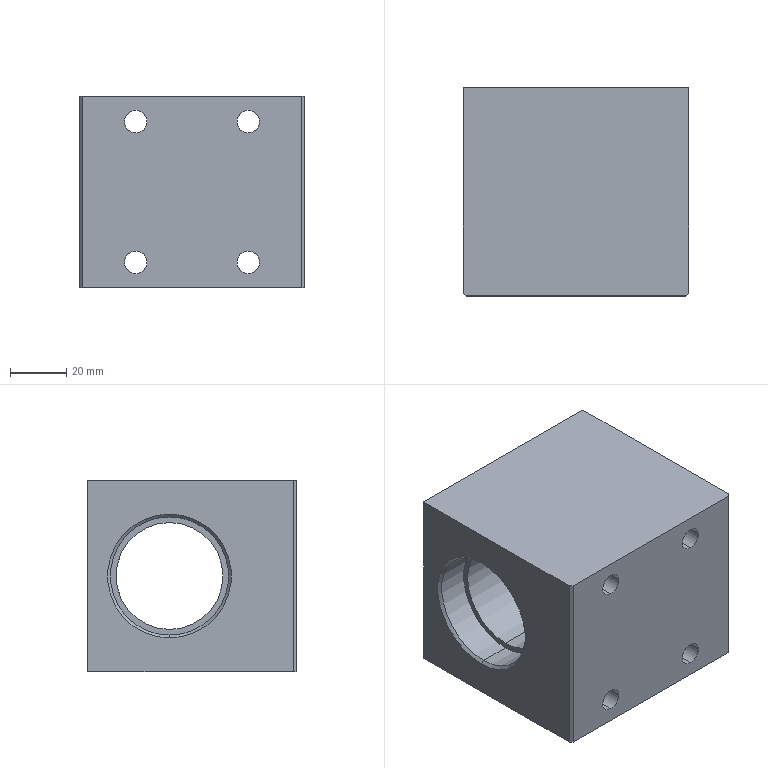Part | SolidWorks | features MirrorPattern 3, Chamfer 2, HoleWzd 2, ICE 2, Extrusion 1, MirrorSolid 1 | 1 solid | 42 faces | box 80 x 74 x 68 mm | volume 288342 mm3 | cylinder 24 | plane 14 | cone 4 | commonest cylinder face diameters 8 x8 12 x8 42 x4 6.8 x2 38 x2
STEP:
#1=CARTESIAN_POINT('',(20.,29.,19.));
#2=VERTEX_POINT('',#1);
#3=CARTESIAN_POINT('',(20.,29.,31.));
#4=VERTEX_POINT('',#3);
#5=CARTESIAN_POINT('',(20.,29.,25.));
#6=DIRECTION('',(0.,1.,0.));
#7=DIRECTION('',(0.,0.,1.));
#8=AXIS2_PLACEMENT_3D('',#5,#6,#7);
#9=CIRCLE('',#8,6.);
#10=EDGE_CURVE('',#2,#4,#9,.T.);
#11=ORIENTED_EDGE('',*,*,#10,.F.);
#12=CARTESIAN_POINT('',(20.,37.,19.));
#13=VERTEX_POINT('',#12);
#14=CARTESIAN_POINT('',(20.,37.,19.));
#15=DIRECTION('',(0.,1.,0.));
#16=VECTOR('',#15,1000.);
#17=LINE('',#14,#16);
#18=EDGE_CURVE('',#2,#13,#17,.T.);
#19=ORIENTED_EDGE('',*,*,#18,.T.);
#20=CARTESIAN_POINT('',(20.,37.,31.));
#21=VERTEX_POINT('',#20);
#22=CARTESIAN_POINT('',(20.,37.,25.));
#23=DIRECTION('',(0.,1.,0.));
#24=DIRECTION('',(0.,0.,1.));
#25=AXIS2_PLACEMENT_3D('',#22,#23,#24);
#26=CIRCLE('',#25,6.);
#27=EDGE_CURVE('',#13,#21,#26,.T.);
#28=ORIENTED_EDGE('',*,*,#27,.T.);
#29=CARTESIAN_POINT('',(20.,37.,31.));
#30=DIRECTION('',(0.,1.,0.));
#31=VECTOR('',#30,1000.);
#32=LINE('',#29,#31);
#33=EDGE_CURVE('',#4,#21,#32,.T.);
#34=ORIENTED_EDGE('',*,*,#33,.F.);
#35=EDGE_LOOP('',(#11,#19,#28,#34));
#36=FACE_OUTER_BOUND('',#35,.T.);
#37=CARTESIAN_POINT('',(20.,37.,25.));
#38=DIRECTION('',(0.,1.,0.));
#39=DIRECTION('',(0.,0.,1.));
#40=AXIS2_PLACEMENT_3D('',#37,#38,#39);
#41=CYLINDRICAL_SURFACE('',#40,6.);
#42=ADVANCED_FACE('',(#36),#41,.F.);
#43=CARTESIAN_POINT('',(20.,-37.,21.));
#44=VERTEX_POINT('',#43);
#45=CARTESIAN_POINT('',(20.,-37.,29.));
#46=VERTEX_POINT('',#45);
#47=CARTESIAN_POINT('',(20.,-37.,25.));
#48=DIRECTION('',(0.,1.,0.));
#49=DIRECTION('',(0.,0.,1.));
#50=AXIS2_PLACEMENT_3D('',#47,#48,#49);
#51=CIRCLE('',#50,4.);
#52=EDGE_CURVE('',#44,#46,#51,.T.);
#53=ORIENTED_EDGE('',*,*,#52,.F.);
#54=CARTESIAN_POINT('',(20.,29.,21.));
#55=VERTEX_POINT('',#54);
#56=CARTESIAN_POINT('',(20.,37.,21.));
#57=DIRECTION('',(0.,1.,0.));
#58=VECTOR('',#57,1000.);
#59=LINE('',#56,#58);
#60=EDGE_CURVE('',#44,#55,#59,.T.);
#61=ORIENTED_EDGE('',*,*,#60,.T.);
#62=CARTESIAN_POINT('',(20.,29.,29.));
#63=VERTEX_POINT('',#62);
#64=CARTESIAN_POINT('',(20.,29.,25.));
#65=DIRECTION('',(0.,1.,0.));
#66=DIRECTION('',(0.,0.,1.));
#67=AXIS2_PLACEMENT_3D('',#64,#65,#66);
#68=CIRCLE('',#67,4.);
#69=EDGE_CURVE('',#55,#63,#68,.T.);
#70=ORIENTED_EDGE('',*,*,#69,.T.);
#71=CARTESIAN_POINT('',(20.,37.,29.));
#72=DIRECTION('',(0.,1.,0.));
#73=VECTOR('',#72,1000.);
#74=LINE('',#71,#73);
#75=EDGE_CURVE('',#46,#63,#74,.T.);
#76=ORIENTED_EDGE('',*,*,#75,.F.);
#77=EDGE_LOOP('',(#53,#61,#70,#76));
#78=FACE_OUTER_BOUND('',#77,.T.);
#79=CARTESIAN_POINT('',(20.,37.,25.));
#80=DIRECTION('',(0.,1.,0.));
#81=DIRECTION('',(0.,0.,1.));
#82=AXIS2_PLACEMENT_3D('',#79,#80,#81);
#83=CYLINDRICAL_SURFACE('',#82,4.);
#84=ADVANCED_FACE('',(#78),#83,.F.);
#85=CARTESIAN_POINT('',(20.,29.,-31.));
#86=VERTEX_POINT('',#85);
#87=CARTESIAN_POINT('',(20.,29.,-19.));
#88=VERTEX_POINT('',#87);
#89=CARTESIAN_POINT('',(20.,29.,-25.));
#90=DIRECTION('',(0.,1.,0.));
#91=DIRECTION('',(0.,0.,1.));
#92=AXIS2_PLACEMENT_3D('',#89,#90,#91);
#93=CIRCLE('',#92,6.);
#94=EDGE_CURVE('',#86,#88,#93,.T.);
#95=ORIENTED_EDGE('',*,*,#94,.F.);
#96=CARTESIAN_POINT('',(20.,37.,-31.));
#97=VERTEX_POINT('',#96);
#98=CARTESIAN_POINT('',(20.,37.,-31.));
#99=DIRECTION('',(0.,1.,0.));
#100=VECTOR('',#99,1000.);
#101=LINE('',#98,#100);
#102=EDGE_CURVE('',#86,#97,#101,.T.);
#103=ORIENTED_EDGE('',*,*,#102,.T.);
#104=CARTESIAN_POINT('',(20.,37.,-19.));
#105=VERTEX_POINT('',#104);
#106=CARTESIAN_POINT('',(20.,37.,-25.));
#107=DIRECTION('',(0.,1.,0.));
#108=DIRECTION('',(0.,0.,1.));
#109=AXIS2_PLACEMENT_3D('',#106,#107,#108);
#110=CIRCLE('',#109,6.);
#111=EDGE_CURVE('',#97,#105,#110,.T.);
#112=ORIENTED_EDGE('',*,*,#111,.T.);
#113=CARTESIAN_POINT('',(20.,37.,-19.));
#114=DIRECTION('',(0.,1.,0.));
#115=VECTOR('',#114,1000.);
#116=LINE('',#113,#115);
#117=EDGE_CURVE('',#88,#105,#116,.T.);
#118=ORIENTED_EDGE('',*,*,#117,.F.);
#119=EDGE_LOOP('',(#95,#103,#112,#118));
#120=FACE_OUTER_BOUND('',#119,.T.);
#121=CARTESIAN_POINT('',(20.,37.,-25.));
#122=DIRECTION('',(0.,1.,0.));
#123=DIRECTION('',(0.,0.,1.));
#124=AXIS2_PLACEMENT_3D('',#121,#122,#123);
#125=CYLINDRICAL_SURFACE('',#124,6.);
#126=ADVANCED_FACE('',(#120),#125,.F.);
#127=CARTESIAN_POINT('',(20.,-37.,-29.));
#128=VERTEX_POINT('',#127);
#129=CARTESIAN_POINT('',(20.,-37.,-21.));
#130=VERTEX_POINT('',#129);
#131=CARTESIAN_POINT('',(20.,-37.,-25.));
#132=DIRECTION('',(0.,1.,0.));
#133=DIRECTION('',(0.,0.,1.));
#134=AXIS2_PLACEMENT_3D('',#131,#132,#133);
#135=CIRCLE('',#134,4.);
#136=EDGE_CURVE('',#128,#130,#135,.T.);
#137=ORIENTED_EDGE('',*,*,#136,.F.);
#138=CARTESIAN_POINT('',(20.,29.,-29.));
#139=VERTEX_POINT('',#138);
#140=CARTESIAN_POINT('',(20.,37.,-29.));
#141=DIRECTION('',(0.,1.,0.));
#142=VECTOR('',#141,1000.);
#143=LINE('',#140,#142);
#144=EDGE_CURVE('',#128,#139,#143,.T.);
#145=ORIENTED_EDGE('',*,*,#144,.T.);
#146=CARTESIAN_POINT('',(20.,29.,-21.));
#147=VERTEX_POINT('',#146);
#148=CARTESIAN_POINT('',(20.,29.,-25.));
#149=DIRECTION('',(0.,1.,0.));
#150=DIRECTION('',(0.,0.,1.));
#151=AXIS2_PLACEMENT_3D('',#148,#149,#150);
#152=CIRCLE('',#151,4.);
#153=EDGE_CURVE('',#139,#147,#152,.T.);
#154=ORIENTED_EDGE('',*,*,#153,.T.);
#155=CARTESIAN_POINT('',(20.,37.,-21.));
#156=DIRECTION('',(0.,1.,0.));
#157=VECTOR('',#156,1000.);
#158=LINE('',#155,#157);
#159=EDGE_CURVE('',#130,#147,#158,.T.);
#160=ORIENTED_EDGE('',*,*,#159,.F.);
#161=EDGE_LOOP('',(#137,#145,#154,#160));
#162=FACE_OUTER_BOUND('',#161,.T.);
#163=CARTESIAN_POINT('',(20.,37.,-25.));
#164=DIRECTION('',(0.,1.,0.));
#165=DIRECTION('',(0.,0.,1.));
#166=AXIS2_PLACEMENT_3D('',#163,#164,#165);
#167=CYLINDRICAL_SURFACE('',#166,4.);
#168=ADVANCED_FACE('',(#162),#167,.F.);
#169=CARTESIAN_POINT('',(-20.,29.,-31.));
#170=VERTEX_POINT('',#169);
#171=CARTESIAN_POINT('',(-20.,29.,-19.));
#172=VERTEX_POINT('',#171);
#173=CARTESIAN_POINT('',(-20.,29.,-25.));
#174=DIRECTION('',(0.,1.,0.));
#175=DIRECTION('',(0.,0.,1.));
#176=AXIS2_PLACEMENT_3D('',#173,#174,#175);
#177=CIRCLE('',#176,6.);
#178=EDGE_CURVE('',#170,#172,#177,.T.);
#179=ORIENTED_EDGE('',*,*,#178,.F.);
#180=CARTESIAN_POINT('',(-20.,37.,-31.));
#181=VERTEX_POINT('',#180);
#182=CARTESIAN_POINT('',(-20.,37.,-31.));
#183=DIRECTION('',(0.,1.,0.));
#184=VECTOR('',#183,1000.);
#185=LINE('',#182,#184);
#186=EDGE_CURVE('',#170,#181,#185,.T.);
#187=ORIENTED_EDGE('',*,*,#186,.T.);
#188=CARTESIAN_POINT('',(-20.,37.,-19.));
#189=VERTEX_POINT('',#188);
#190=CARTESIAN_POINT('',(-20.,37.,-25.));
#191=DIRECTION('',(0.,1.,0.));
#192=DIRECTION('',(0.,0.,1.));
#193=AXIS2_PLACEMENT_3D('',#190,#191,#192);
#194=CIRCLE('',#193,6.);
#195=EDGE_CURVE('',#181,#189,#194,.T.);
#196=ORIENTED_EDGE('',*,*,#195,.T.);
#197=CARTESIAN_POINT('',(-20.,37.,-19.));
#198=DIRECTION('',(0.,1.,0.));
#199=VECTOR('',#198,1000.);
#200=LINE('',#197,#199);
#201=EDGE_CURVE('',#172,#189,#200,.T.);
#202=ORIENTED_EDGE('',*,*,#201,.F.);
#203=EDGE_LOOP('',(#179,#187,#196,#202));
#204=FACE_OUTER_BOUND('',#203,.T.);
#205=CARTESIAN_POINT('',(-20.,37.,-25.));
#206=DIRECTION('',(0.,1.,0.));
#207=DIRECTION('',(0.,0.,1.));
#208=AXIS2_PLACEMENT_3D('',#205,#206,#207);
#209=CYLINDRICAL_SURFACE('',#208,6.);
#210=ADVANCED_FACE('',(#204),#209,.F.);
#211=CARTESIAN_POINT('',(-20.,-37.,-29.));
#212=VERTEX_POINT('',#211);
#213=CARTESIAN_POINT('',(-20.,-37.,-21.));
#214=VERTEX_POINT('',#213);
#215=CARTESIAN_POINT('',(-20.,-37.,-25.));
#216=DIRECTION('',(0.,1.,0.));
#217=DIRECTION('',(0.,0.,1.));
#218=AXIS2_PLACEMENT_3D('',#215,#216,#217);
#219=CIRCLE('',#218,4.);
#220=EDGE_CURVE('',#212,#214,#219,.T.);
#221=ORIENTED_EDGE('',*,*,#220,.F.);
#222=CARTESIAN_POINT('',(-20.,29.,-29.));
#223=VERTEX_POINT('',#222);
#224=CARTESIAN_POINT('',(-20.,37.,-29.));
#225=DIRECTION('',(0.,1.,0.));
#226=VECTOR('',#225,1000.);
#227=LINE('',#224,#226);
#228=EDGE_CURVE('',#212,#223,#227,.T.);
#229=ORIENTED_EDGE('',*,*,#228,.T.);
#230=CARTESIAN_POINT('',(-20.,29.,-21.));
#231=VERTEX_POINT('',#230);
#232=CARTESIAN_POINT('',(-20.,29.,-25.));
#233=DIRECTION('',(0.,1.,0.));
#234=DIRECTION('',(0.,0.,1.));
#235=AXIS2_PLACEMENT_3D('',#232,#233,#234);
#236=CIRCLE('',#235,4.);
#237=EDGE_CURVE('',#223,#231,#236,.T.);
#238=ORIENTED_EDGE('',*,*,#237,.T.);
#239=CARTESIAN_POINT('',(-20.,37.,-21.));
#240=DIRECTION('',(0.,1.,0.));
#241=VECTOR('',#240,1000.);
#242=LINE('',#239,#241);
#243=EDGE_CURVE('',#214,#231,#242,.T.);
#244=ORIENTED_EDGE('',*,*,#243,.F.);
#245=EDGE_LOOP('',(#221,#229,#238,#244));
#246=FACE_OUTER_BOUND('',#245,.T.);
#247=CARTESIAN_POINT('',(-20.,37.,-25.));
#248=DIRECTION('',(0.,1.,0.));
#249=DIRECTION('',(0.,0.,1.));
#250=AXIS2_PLACEMENT_3D('',#247,#248,#249);
#251=CYLINDRICAL_SURFACE('',#250,4.);
#252=ADVANCED_FACE('',(#246),#251,.F.);
#253=CARTESIAN_POINT('',(-20.,29.,19.));
#254=VERTEX_POINT('',#253);
#255=CARTESIAN_POINT('',(-20.,29.,31.));
#256=VERTEX_POINT('',#255);
#257=CARTESIAN_POINT('',(-20.,29.,25.));
#258=DIRECTION('',(0.,1.,0.));
#259=DIRECTION('',(0.,0.,1.));
#260=AXIS2_PLACEMENT_3D('',#257,#258,#259);
#261=CIRCLE('',#260,6.);
#262=EDGE_CURVE('',#254,#256,#261,.T.);
#263=ORIENTED_EDGE('',*,*,#262,.F.);
#264=CARTESIAN_POINT('',(-20.,37.,19.));
#265=VERTEX_POINT('',#264);
#266=CARTESIAN_POINT('',(-20.,37.,19.));
#267=DIRECTION('',(0.,1.,0.));
#268=VECTOR('',#267,1000.);
#269=LINE('',#266,#268);
#270=EDGE_CURVE('',#254,#265,#269,.T.);
#271=ORIENTED_EDGE('',*,*,#270,.T.);
#272=CARTESIAN_POINT('',(-20.,37.,31.));
#273=VERTEX_POINT('',#272);
#274=CARTESIAN_POINT('',(-20.,37.,25.));
#275=DIRECTION('',(0.,1.,0.));
#276=DIRECTION('',(0.,0.,1.));
#277=AXIS2_PLACEMENT_3D('',#274,#275,#276);
#278=CIRCLE('',#277,6.);
#279=EDGE_CURVE('',#265,#273,#278,.T.);
#280=ORIENTED_EDGE('',*,*,#279,.T.);
#281=CARTESIAN_POINT('',(-20.,37.,31.));
#282=DIRECTION('',(0.,1.,0.));
#283=VECTOR('',#282,1000.);
#284=LINE('',#281,#283);
#285=EDGE_CURVE('',#256,#273,#284,.T.);
#286=ORIENTED_EDGE('',*,*,#285,.F.);
#287=EDGE_LOOP('',(#263,#271,#280,#286));
#288=FACE_OUTER_BOUND('',#287,.T.);
#289=CARTESIAN_POINT('',(-20.,37.,25.));
#290=DIRECTION('',(0.,1.,0.));
#291=DIRECTION('',(0.,0.,1.));
#292=AXIS2_PLACEMENT_3D('',#289,#290,#291);
#293=CYLINDRICAL_SURFACE('',#292,6.);
#294=ADVANCED_FACE('',(#288),#293,.F.);
#295=CARTESIAN_POINT('',(-20.,-37.,21.));
#296=VERTEX_POINT('',#295);
#297=CARTESIAN_POINT('',(-20.,-37.,29.));
#298=VERTEX_POINT('',#297);
#299=CARTESIAN_POINT('',(-20.,-37.,25.));
#300=DIRECTION('',(0.,1.,0.));
#301=DIRECTION('',(0.,0.,1.));
#302=AXIS2_PLACEMENT_3D('',#299,#300,#301);
#303=CIRCLE('',#302,4.);
#304=EDGE_CURVE('',#296,#298,#303,.T.);
#305=ORIENTED_EDGE('',*,*,#304,.F.);
#306=CARTESIAN_POINT('',(-20.,29.,21.));
#307=VERTEX_POINT('',#306);
#308=CARTESIAN_POINT('',(-20.,37.,21.));
#309=DIRECTION('',(0.,1.,0.));
#310=VECTOR('',#309,1000.);
#311=LINE('',#308,#310);
#312=EDGE_CURVE('',#296,#307,#311,.T.);
#313=ORIENTED_EDGE('',*,*,#312,.T.);
#314=CARTESIAN_POINT('',(-20.,29.,29.));
#315=VERTEX_POINT('',#314);
#316=CARTESIAN_POINT('',(-20.,29.,25.));
#317=DIRECTION('',(0.,1.,0.));
#318=DIRECTION('',(0.,0.,1.));
#319=AXIS2_PLACEMENT_3D('',#316,#317,#318);
#320=CIRCLE('',#319,4.);
#321=EDGE_CURVE('',#307,#315,#320,.T.);
#322=ORIENTED_EDGE('',*,*,#321,.T.);
#323=CARTESIAN_POINT('',(-20.,37.,29.));
#324=DIRECTION('',(0.,1.,0.));
#325=VECTOR('',#324,1000.);
#326=LINE('',#323,#325);
#327=EDGE_CURVE('',#298,#315,#326,.T.);
#328=ORIENTED_EDGE('',*,*,#327,.F.);
#329=EDGE_LOOP('',(#305,#313,#322,#328));
#330=FACE_OUTER_BOUND('',#329,.T.);
#331=CARTESIAN_POINT('',(-20.,37.,25.));
#332=DIRECTION('',(0.,1.,0.));
#333=DIRECTION('',(0.,0.,1.));
#334=AXIS2_PLACEMENT_3D('',#331,#332,#333);
#335=CYLINDRICAL_SURFACE('',#334,4.);
#336=ADVANCED_FACE('',(#330),#335,.F.);
#337=CARTESIAN_POINT('',(39.,8.,21.));
#338=VERTEX_POINT('',#337);
#339=CARTESIAN_POINT('',(39.,8.,-21.));
#340=VERTEX_POINT('',#339);
#341=CARTESIAN_POINT('',(39.,8.,0.));
#342=DIRECTION('',(1.,0.,0.));
#343=DIRECTION('',(0.,0.,1.));
#344=AXIS2_PLACEMENT_3D('',#341,#342,#343);
#345=CIRCLE('',#344,21.);
#346=EDGE_CURVE('',#338,#340,#345,.T.);
#347=ORIENTED_EDGE('',*,*,#346,.F.);
#348=CARTESIAN_POINT('',(40.,8.,22.));
#349=VERTEX_POINT('',#348);
#350=CARTESIAN_POINT('',(39.,8.,21.));
#351=DIRECTION('',(0.7071,0.,0.7071));
#352=VECTOR('',#351,1000.);
#353=LINE('',#350,#352);
#354=EDGE_CURVE('',#338,#349,#353,.T.);
#355=ORIENTED_EDGE('',*,*,#354,.T.);
#356=CARTESIAN_POINT('',(40.,8.,-22.));
#357=VERTEX_POINT('',#356);
#358=CARTESIAN_POINT('',(40.,8.,0.));
#359=DIRECTION('',(-1.,0.,0.));
#360=DIRECTION('',(0.,0.,1.));
#361=AXIS2_PLACEMENT_3D('',#358,#359,#360);
#362=CIRCLE('',#361,22.);
#363=EDGE_CURVE('',#357,#349,#362,.T.);
#364=ORIENTED_EDGE('',*,*,#363,.F.);
#365=CARTESIAN_POINT('',(39.,8.,-21.));
#366=DIRECTION('',(0.7071,0.,-0.7071));
#367=VECTOR('',#366,1000.);
#368=LINE('',#365,#367);
#369=EDGE_CURVE('',#340,#357,#368,.T.);
#370=ORIENTED_EDGE('',*,*,#369,.F.);
#371=EDGE_LOOP('',(#347,#355,#364,#370));
#372=FACE_OUTER_BOUND('',#371,.T.);
#373=CARTESIAN_POINT('',(39.,8.,0.));
#374=DIRECTION('',(1.,0.,0.));
#375=DIRECTION('',(0.,0.,-1.));
#376=AXIS2_PLACEMENT_3D('',#373,#374,#375);
#377=CONICAL_SURFACE('',#376,21.,0.7854);
#378=ADVANCED_FACE('',(#372),#377,.F.);
#379=CARTESIAN_POINT('',(-39.,8.,-21.));
#380=VERTEX_POINT('',#379);
#381=CARTESIAN_POINT('',(-39.,8.,21.));
#382=VERTEX_POINT('',#381);
#383=CARTESIAN_POINT('',(-39.,8.,0.));
#384=DIRECTION('',(-1.,0.,0.));
#385=DIRECTION('',(0.,0.,-1.));
#386=AXIS2_PLACEMENT_3D('',#383,#384,#385);
#387=CIRCLE('',#386,21.);
#388=EDGE_CURVE('',#380,#382,#387,.T.);
#389=ORIENTED_EDGE('',*,*,#388,.F.);
#390=CARTESIAN_POINT('',(-40.,8.,-22.));
#391=VERTEX_POINT('',#390);
#392=CARTESIAN_POINT('',(-40.,8.,-22.));
#393=DIRECTION('',(-0.7071,0.,-0.7071));
#394=VECTOR('',#393,1000.);
#395=LINE('',#392,#394);
#396=EDGE_CURVE('',#380,#391,#395,.T.);
#397=ORIENTED_EDGE('',*,*,#396,.T.);
#398=CARTESIAN_POINT('',(-40.,8.,22.));
#399=VERTEX_POINT('',#398);
#400=CARTESIAN_POINT('',(-40.,8.,0.));
#401=DIRECTION('',(1.,0.,0.));
#402=DIRECTION('',(0.,0.,-1.));
#403=AXIS2_PLACEMENT_3D('',#400,#401,#402);
#404=CIRCLE('',#403,22.);
#405=EDGE_CURVE('',#399,#391,#404,.T.);
#406=ORIENTED_EDGE('',*,*,#405,.F.);
#407=CARTESIAN_POINT('',(-40.,8.,22.));
#408=DIRECTION('',(-0.7071,0.,0.7071));
#409=VECTOR('',#408,1000.);
#410=LINE('',#407,#409);
#411=EDGE_CURVE('',#382,#399,#410,.T.);
#412=ORIENTED_EDGE('',*,*,#411,.F.);
#413=EDGE_LOOP('',(#389,#397,#406,#412));
#414=FACE_OUTER_BOUND('',#413,.T.);
#415=CARTESIAN_POINT('',(-40.,8.,0.));
#416=DIRECTION('',(-1.,0.,0.));
#417=DIRECTION('',(0.,0.,1.));
#418=AXIS2_PLACEMENT_3D('',#415,#416,#417);
#419=CONICAL_SURFACE('',#418,22.,0.7854);
#420=ADVANCED_FACE('',(#414),#419,.F.);
#421=CARTESIAN_POINT('',(-28.,8.,-19.));
#422=VERTEX_POINT('',#421);
#423=CARTESIAN_POINT('',(-28.,8.,19.));
#424=VERTEX_POINT('',#423);
#425=CARTESIAN_POINT('',(-28.,8.,0.));
#426=DIRECTION('',(-1.,0.,0.));
#427=DIRECTION('',(0.,0.,1.));
#428=AXIS2_PLACEMENT_3D('',#425,#426,#427);
#429=CIRCLE('',#428,19.);
#430=EDGE_CURVE('',#422,#424,#429,.T.);
#431=ORIENTED_EDGE('',*,*,#430,.T.);
#432=CARTESIAN_POINT('',(28.,8.,19.));
#433=VERTEX_POINT('',#432);
#434=CARTESIAN_POINT('',(-40.,8.,19.));
#435=DIRECTION('',(1.,0.,0.));
#436=VECTOR('',#435,1000.);
#437=LINE('',#434,#436);
#438=EDGE_CURVE('',#424,#433,#437,.T.);
#439=ORIENTED_EDGE('',*,*,#438,.T.);
#440=CARTESIAN_POINT('',(28.,8.,-19.));
#441=VERTEX_POINT('',#440);
#442=CARTESIAN_POINT('',(28.,8.,0.));
#443=DIRECTION('',(1.,0.,0.));
#444=DIRECTION('',(0.,0.,-1.));
#445=AXIS2_PLACEMENT_3D('',#442,#443,#444);
#446=CIRCLE('',#445,19.);
#447=EDGE_CURVE('',#433,#441,#446,.T.);
#448=ORIENTED_EDGE('',*,*,#447,.T.);
#449=CARTESIAN_POINT('',(-40.,8.,-19.));
#450=DIRECTION('',(1.,0.,0.));
#451=VECTOR('',#450,1000.);
#452=LINE('',#449,#451);
#453=EDGE_CURVE('',#422,#441,#452,.T.);
#454=ORIENTED_EDGE('',*,*,#453,.F.);
#455=EDGE_LOOP('',(#431,#439,#448,#454));
#456=FACE_OUTER_BOUND('',#455,.T.);
#457=CARTESIAN_POINT('',(-40.,8.,0.));
#458=DIRECTION('',(1.,0.,0.));
#459=DIRECTION('',(0.,0.,-1.));
#460=AXIS2_PLACEMENT_3D('',#457,#458,#459);
#461=CYLINDRICAL_SURFACE('',#460,19.);
#462=ADVANCED_FACE('',(#456),#461,.F.);
#463=CARTESIAN_POINT('',(-28.,8.,21.));
#464=VERTEX_POINT('',#463);
#465=CARTESIAN_POINT('',(-28.,8.,-21.));
#466=VERTEX_POINT('',#465);
#467=CARTESIAN_POINT('',(-28.,8.,0.));
#468=DIRECTION('',(1.,0.,0.));
#469=DIRECTION('',(0.,0.,-1.));
#470=AXIS2_PLACEMENT_3D('',#467,#468,#469);
#471=CIRCLE('',#470,21.);
#472=EDGE_CURVE('',#464,#466,#471,.T.);
#473=ORIENTED_EDGE('',*,*,#472,.T.);
#474=CARTESIAN_POINT('',(-28.,8.,-21.));
#475=DIRECTION('',(-1.,0.,0.));
#476=VECTOR('',#475,1000.);
#477=LINE('',#474,#476);
#478=EDGE_CURVE('',#466,#380,#477,.T.);
#479=ORIENTED_EDGE('',*,*,#478,.T.);
#480=ORIENTED_EDGE('',*,*,#388,.T.);
#481=CARTESIAN_POINT('',(-28.,8.,21.));
#482=DIRECTION('',(-1.,0.,0.));
#483=VECTOR('',#482,1000.);
#484=LINE('',#481,#483);
#485=EDGE_CURVE('',#464,#382,#484,.T.);
#486=ORIENTED_EDGE('',*,*,#485,.F.);
#487=EDGE_LOOP('',(#473,#479,#480,#486));
#488=FACE_OUTER_BOUND('',#487,.T.);
#489=CARTESIAN_POINT('',(-28.,8.,0.));
#490=DIRECTION('',(-1.,0.,0.));
#491=DIRECTION('',(0.,0.,1.));
#492=AXIS2_PLACEMENT_3D('',#489,#490,#491);
#493=CYLINDRICAL_SURFACE('',#492,21.);
#494=ADVANCED_FACE('',(#488),#493,.F.);
#495=CARTESIAN_POINT('',(28.,8.,21.));
#496=VERTEX_POINT('',#495);
#497=CARTESIAN_POINT('',(28.,8.,-21.));
#498=VERTEX_POINT('',#497);
#499=CARTESIAN_POINT('',(28.,8.,0.));
#500=DIRECTION('',(1.,0.,0.));
#501=DIRECTION('',(0.,0.,-1.));
#502=AXIS2_PLACEMENT_3D('',#499,#500,#501);
#503=CIRCLE('',#502,21.);
#504=EDGE_CURVE('',#496,#498,#503,.T.);
#505=ORIENTED_EDGE('',*,*,#504,.F.);
#506=CARTESIAN_POINT('',(28.,8.,21.));
#507=DIRECTION('',(1.,0.,0.));
#508=VECTOR('',#507,1000.);
#509=LINE('',#506,#508);
#510=EDGE_CURVE('',#496,#338,#509,.T.);
#511=ORIENTED_EDGE('',*,*,#510,.T.);
#512=ORIENTED_EDGE('',*,*,#346,.T.);
#513=CARTESIAN_POINT('',(28.,8.,-21.));
#514=DIRECTION('',(1.,0.,0.));
#515=VECTOR('',#514,1000.);
#516=LINE('',#513,#515);
#517=EDGE_CURVE('',#498,#340,#516,.T.);
#518=ORIENTED_EDGE('',*,*,#517,.F.);
#519=EDGE_LOOP('',(#505,#511,#512,#518));
#520=FACE_OUTER_BOUND('',#519,.T.);
#521=CARTESIAN_POINT('',(28.,8.,0.));
#522=DIRECTION('',(1.,0.,0.));
#523=DIRECTION('',(0.,0.,-1.));
#524=AXIS2_PLACEMENT_3D('',#521,#522,#523);
#525=CYLINDRICAL_SURFACE('',#524,21.);
#526=ADVANCED_FACE('',(#520),#525,.F.);
#527=CARTESIAN_POINT('',(0.,26.693,3.4));
#528=VERTEX_POINT('',#527);
#529=CARTESIAN_POINT('',(0.,26.693,-3.4));
#530=VERTEX_POINT('',#529);
#531=CARTESIAN_POINT('',(0.,26.693,3.4));
#532=CARTESIAN_POINT('',(-0.2251,26.693,3.4));
#533=CARTESIAN_POINT('',(-0.4464,26.697,3.378));
#534=CARTESIAN_POINT('',(-0.8816,26.713,3.291));
#535=CARTESIAN_POINT('',(-1.098,26.724,3.226));
#536=CARTESIAN_POINT('',(-1.509,26.753,3.055));
#537=CARTESIAN_POINT('',(-1.704,26.77,2.95));
#538=CARTESIAN_POINT('',(-2.074,26.807,2.703));
#539=CARTESIAN_POINT('',(-2.248,26.827,2.56));
#540=CARTESIAN_POINT('',(-2.561,26.867,2.247));
#541=CARTESIAN_POINT('',(-2.702,26.887,2.076));
#542=CARTESIAN_POINT('',(-2.95,26.924,1.705));
#543=CARTESIAN_POINT('',(-3.056,26.941,1.507));
#544=CARTESIAN_POINT('',(-3.225,26.969,1.098));
#545=CARTESIAN_POINT('',(-3.291,26.981,0.8836));
#546=CARTESIAN_POINT('',(-3.378,26.996,0.4445));
#547=CARTESIAN_POINT('',(-3.4,27.,0.2236));
#548=CARTESIAN_POINT('',(-3.4,27.,-0.221));
#549=CARTESIAN_POINT('',(-3.378,26.996,-0.4468));
#550=CARTESIAN_POINT('',(-3.291,26.981,-0.8832));
#551=CARTESIAN_POINT('',(-3.226,26.97,-1.095));
#552=CARTESIAN_POINT('',(-3.056,26.941,-1.508));
#553=CARTESIAN_POINT('',(-2.949,26.924,-1.706));
#554=CARTESIAN_POINT('',(-2.703,26.887,-2.074));
#555=CARTESIAN_POINT('',(-2.562,26.867,-2.246));
#556=CARTESIAN_POINT('',(-2.246,26.827,-2.562));
#557=CARTESIAN_POINT('',(-2.075,26.807,-2.703));
#558=CARTESIAN_POINT('',(-1.707,26.77,-2.949));
#559=CARTESIAN_POINT('',(-1.508,26.753,-3.056));
#560=CARTESIAN_POINT('',(-1.096,26.724,-3.226));
#561=CARTESIAN_POINT('',(-0.8845,26.713,-3.29));
#562=CARTESIAN_POINT('',(-0.4478,26.697,-3.378));
#563=CARTESIAN_POINT('',(-0.2221,26.693,-3.4));
#564=CARTESIAN_POINT('',(0.,26.693,-3.4));
#565=B_SPLINE_CURVE_WITH_KNOTS('',3,(#531,#532,#533,#534,#535,#536,#537,#538,#539,#540,#541,#542,#543,#544,#545,#546,#547,#548,#549,#550,#551,#552,#553,#554,#555,#556,#557,#558,#559,#560,#561,#562,#563,#564),.UNSPECIFIED.,.F.,.F.,(4,2,2,2,2,2,2,2,2,2,2,2,2,2,2,2,4),(0.,0.0006657,0.001331,0.001997,0.002663,0.003329,0.003994,0.00466,0.005326,0.005991,0.006657,0.007323,0.007989,0.008654,0.00932,0.009986,0.01065),.UNSPECIFIED.);
#566=EDGE_CURVE('',#528,#530,#565,.T.);
#567=ORIENTED_EDGE('',*,*,#566,.T.);
#568=CARTESIAN_POINT('',(0.,37.,-3.4));
#569=VERTEX_POINT('',#568);
#570=CARTESIAN_POINT('',(0.,37.,-3.4));
#571=DIRECTION('',(0.,1.,0.));
#572=VECTOR('',#571,1000.);
#573=LINE('',#570,#572);
#574=EDGE_CURVE('',#530,#569,#573,.T.);
#575=ORIENTED_EDGE('',*,*,#574,.T.);
#576=CARTESIAN_POINT('',(0.,37.,3.4));
#577=VERTEX_POINT('',#576);
#578=CARTESIAN_POINT('',(0.,37.,0.));
#579=DIRECTION('',(0.,1.,0.));
#580=DIRECTION('',(0.,0.,1.));
#581=AXIS2_PLACEMENT_3D('',#578,#579,#580);
#582=CIRCLE('',#581,3.4);
#583=EDGE_CURVE('',#569,#577,#582,.T.);
#584=ORIENTED_EDGE('',*,*,#583,.T.);
#585=CARTESIAN_POINT('',(0.,37.,3.4));
#586=DIRECTION('',(0.,1.,0.));
#587=VECTOR('',#586,1000.);
#588=LINE('',#585,#587);
#589=EDGE_CURVE('',#528,#577,#588,.T.);
#590=ORIENTED_EDGE('',*,*,#589,.F.);
#591=EDGE_LOOP('',(#567,#575,#584,#590));
#592=FACE_OUTER_BOUND('',#591,.T.);
#593=CARTESIAN_POINT('',(0.,37.,0.));
#594=DIRECTION('',(0.,1.,0.));
#595=DIRECTION('',(0.,0.,1.));
#596=AXIS2_PLACEMENT_3D('',#593,#594,#595);
#597=CYLINDRICAL_SURFACE('',#596,3.4);
#598=ADVANCED_FACE('',(#592),#597,.F.);
#599=CARTESIAN_POINT('',(-40.,37.,34.));
#600=VERTEX_POINT('',#599);
#601=CARTESIAN_POINT('',(-40.,-36.,34.));
#602=VERTEX_POINT('',#601);
#603=CARTESIAN_POINT('',(-40.,37.,34.));
#604=DIRECTION('',(0.,-1.,0.));
#605=VECTOR('',#604,1000.);
#606=LINE('',#603,#605);
#607=EDGE_CURVE('',#600,#602,#606,.T.);
#608=ORIENTED_EDGE('',*,*,#607,.T.);
#609=CARTESIAN_POINT('',(-39.,-37.,34.));
#610=VERTEX_POINT('',#609);
#611=CARTESIAN_POINT('',(-39.,-37.,34.));
#612=DIRECTION('',(0.7071,-0.7071,0.));
#613=VECTOR('',#612,1000.);
#614=LINE('',#611,#613);
#615=EDGE_CURVE('',#602,#610,#614,.T.);
#616=ORIENTED_EDGE('',*,*,#615,.T.);
#617=CARTESIAN_POINT('',(39.,-37.,34.));
#618=VERTEX_POINT('',#617);
#619=CARTESIAN_POINT('',(0.,-37.,34.));
#620=DIRECTION('',(1.,0.,0.));
#621=VECTOR('',#620,1000.);
#622=LINE('',#619,#621);
#623=EDGE_CURVE('',#610,#618,#622,.T.);
#624=ORIENTED_EDGE('',*,*,#623,.T.);
#625=CARTESIAN_POINT('',(40.,-36.,34.));
#626=VERTEX_POINT('',#625);
#627=CARTESIAN_POINT('',(40.,-36.,34.));
#628=DIRECTION('',(0.7071,0.7071,0.));
#629=VECTOR('',#628,1000.);
#630=LINE('',#627,#629);
#631=EDGE_CURVE('',#618,#626,#630,.T.);
#632=ORIENTED_EDGE('',*,*,#631,.T.);
#633=CARTESIAN_POINT('',(40.,37.,34.));
#634=VERTEX_POINT('',#633);
#635=CARTESIAN_POINT('',(40.,37.,34.));
#636=DIRECTION('',(0.,-1.,0.));
#637=VECTOR('',#636,1000.);
#638=LINE('',#635,#637);
#639=EDGE_CURVE('',#634,#626,#638,.T.);
#640=ORIENTED_EDGE('',*,*,#639,.F.);
#641=CARTESIAN_POINT('',(0.,37.,34.));
#642=DIRECTION('',(1.,0.,0.));
#643=VECTOR('',#642,1000.);
#644=LINE('',#641,#643);
#645=EDGE_CURVE('',#600,#634,#644,.T.);
#646=ORIENTED_EDGE('',*,*,#645,.F.);
#647=EDGE_LOOP('',(#608,#616,#624,#632,#640,#646));
#648=FACE_OUTER_BOUND('',#647,.T.);
#649=CARTESIAN_POINT('',(0.,37.,34.));
#650=DIRECTION('',(0.,0.,-1.));
#651=DIRECTION('',(-1.,0.,0.));
#652=AXIS2_PLACEMENT_3D('',#649,#650,#651);
#653=PLANE('',#652);
#654=ADVANCED_FACE('',(#648),#653,.F.);
#655=ORIENTED_EDGE('',*,*,#363,.T.);
#656=CARTESIAN_POINT('',(40.,8.,0.));
#657=DIRECTION('',(-1.,0.,0.));
#658=DIRECTION('',(0.,0.,1.));
#659=AXIS2_PLACEMENT_3D('',#656,#657,#658);
#660=CIRCLE('',#659,22.);
#661=EDGE_CURVE('',#349,#357,#660,.T.);
#662=ORIENTED_EDGE('',*,*,#661,.T.);
#663=EDGE_LOOP('',(#655,#662));
#664=FACE_BOUND('',#663,.T.);
#665=ORIENTED_EDGE('',*,*,#639,.T.);
#666=CARTESIAN_POINT('',(40.,-36.,-34.));
#667=VERTEX_POINT('',#666);
#668=CARTESIAN_POINT('',(40.,-36.,0.));
#669=DIRECTION('',(0.,0.,-1.));
#670=VECTOR('',#669,1000.);
#671=LINE('',#668,#670);
#672=EDGE_CURVE('',#626,#667,#671,.T.);
#673=ORIENTED_EDGE('',*,*,#672,.T.);
#674=CARTESIAN_POINT('',(40.,37.,-34.));
#675=VERTEX_POINT('',#674);
#676=CARTESIAN_POINT('',(40.,37.,-34.));
#677=DIRECTION('',(0.,-1.,0.));
#678=VECTOR('',#677,1000.);
#679=LINE('',#676,#678);
#680=EDGE_CURVE('',#675,#667,#679,.T.);
#681=ORIENTED_EDGE('',*,*,#680,.F.);
#682=CARTESIAN_POINT('',(40.,37.,0.));
#683=DIRECTION('',(0.,0.,-1.));
#684=VECTOR('',#683,1000.);
#685=LINE('',#682,#684);
#686=EDGE_CURVE('',#634,#675,#685,.T.);
#687=ORIENTED_EDGE('',*,*,#686,.F.);
#688=EDGE_LOOP('',(#665,#673,#681,#687));
#689=FACE_OUTER_BOUND('',#688,.T.);
#690=CARTESIAN_POINT('',(40.,37.,0.));
#691=DIRECTION('',(-1.,0.,0.));
#692=DIRECTION('',(0.,0.,1.));
#693=AXIS2_PLACEMENT_3D('',#690,#691,#692);
#694=PLANE('',#693);
#695=ADVANCED_FACE('',(#664,#689),#694,.F.);
#696=CARTESIAN_POINT('',(-39.,-37.,-34.));
#697=VERTEX_POINT('',#696);
#698=CARTESIAN_POINT('',(39.,-37.,-34.));
#699=VERTEX_POINT('',#698);
#700=CARTESIAN_POINT('',(0.,-37.,-34.));
#701=DIRECTION('',(1.,0.,0.));
#702=VECTOR('',#701,1000.);
#703=LINE('',#700,#702);
#704=EDGE_CURVE('',#697,#699,#703,.T.);
#705=ORIENTED_EDGE('',*,*,#704,.F.);
#706=CARTESIAN_POINT('',(-40.,-36.,-34.));
#707=VERTEX_POINT('',#706);
#708=CARTESIAN_POINT('',(-56.5,-19.5,-34.));
#709=DIRECTION('',(-0.7071,0.7071,0.));
#710=VECTOR('',#709,1000.);
#711=LINE('',#708,#710);
#712=EDGE_CURVE('',#697,#707,#711,.T.);
#713=ORIENTED_EDGE('',*,*,#712,.T.);
#714=CARTESIAN_POINT('',(-40.,37.,-34.));
#715=VERTEX_POINT('',#714);
#716=CARTESIAN_POINT('',(-40.,37.,-34.));
#717=DIRECTION('',(0.,-1.,0.));
#718=VECTOR('',#717,1000.);
#719=LINE('',#716,#718);
#720=EDGE_CURVE('',#715,#707,#719,.T.);
#721=ORIENTED_EDGE('',*,*,#720,.F.);
#722=CARTESIAN_POINT('',(0.,37.,-34.));
#723=DIRECTION('',(1.,0.,0.));
#724=VECTOR('',#723,1000.);
#725=LINE('',#722,#724);
#726=EDGE_CURVE('',#715,#675,#725,.T.);
#727=ORIENTED_EDGE('',*,*,#726,.T.);
#728=ORIENTED_EDGE('',*,*,#680,.T.);
#729=CARTESIAN_POINT('',(56.5,-19.5,-34.));
#730=DIRECTION('',(-0.7071,-0.7071,0.));
#731=VECTOR('',#730,1000.);
#732=LINE('',#729,#731);
#733=EDGE_CURVE('',#667,#699,#732,.T.);
#734=ORIENTED_EDGE('',*,*,#733,.T.);
#735=EDGE_LOOP('',(#705,#713,#721,#727,#728,#734));
#736=FACE_OUTER_BOUND('',#735,.T.);
#737=CARTESIAN_POINT('',(0.,37.,-34.));
#738=DIRECTION('',(0.,0.,-1.));
#739=DIRECTION('',(-1.,0.,0.));
#740=AXIS2_PLACEMENT_3D('',#737,#738,#739);
#741=PLANE('',#740);
#742=ADVANCED_FACE('',(#736),#741,.T.);
#743=CARTESIAN_POINT('',(20.,37.,25.));
#744=DIRECTION('',(0.,1.,0.));
#745=DIRECTION('',(0.,0.,1.));
#746=AXIS2_PLACEMENT_3D('',#743,#744,#745);
#747=CIRCLE('',#746,6.);
#748=EDGE_CURVE('',#21,#13,#747,.T.);
#749=ORIENTED_EDGE('',*,*,#748,.F.);
#750=ORIENTED_EDGE('',*,*,#27,.F.);
#751=EDGE_LOOP('',(#749,#750));
#752=FACE_BOUND('',#751,.T.);
#753=CARTESIAN_POINT('',(20.,37.,-25.));
#754=DIRECTION('',(0.,1.,0.));
#755=DIRECTION('',(0.,0.,1.));
#756=AXIS2_PLACEMENT_3D('',#753,#754,#755);
#757=CIRCLE('',#756,6.);
#758=EDGE_CURVE('',#105,#97,#757,.T.);
#759=ORIENTED_EDGE('',*,*,#758,.F.);
#760=ORIENTED_EDGE('',*,*,#111,.F.);
#761=EDGE_LOOP('',(#759,#760));
#762=FACE_BOUND('',#761,.T.);
#763=CARTESIAN_POINT('',(-20.,37.,-25.));
#764=DIRECTION('',(0.,1.,0.));
#765=DIRECTION('',(0.,0.,1.));
#766=AXIS2_PLACEMENT_3D('',#763,#764,#765);
#767=CIRCLE('',#766,6.);
#768=EDGE_CURVE('',#189,#181,#767,.T.);
#769=ORIENTED_EDGE('',*,*,#768,.F.);
#770=ORIENTED_EDGE('',*,*,#195,.F.);
#771=EDGE_LOOP('',(#769,#770));
#772=FACE_BOUND('',#771,.T.);
#773=CARTESIAN_POINT('',(-20.,37.,25.));
#774=DIRECTION('',(0.,1.,0.));
#775=DIRECTION('',(0.,0.,1.));
#776=AXIS2_PLACEMENT_3D('',#773,#774,#775);
#777=CIRCLE('',#776,6.);
#778=EDGE_CURVE('',#273,#265,#777,.T.);
#779=ORIENTED_EDGE('',*,*,#778,.F.);
#780=ORIENTED_EDGE('',*,*,#279,.F.);
#781=EDGE_LOOP('',(#779,#780));
#782=FACE_BOUND('',#781,.T.);
#783=CARTESIAN_POINT('',(0.,37.,0.));
#784=DIRECTION('',(0.,1.,0.));
#785=DIRECTION('',(0.,0.,1.));
#786=AXIS2_PLACEMENT_3D('',#783,#784,#785);
#787=CIRCLE('',#786,3.4);
#788=EDGE_CURVE('',#577,#569,#787,.T.);
#789=ORIENTED_EDGE('',*,*,#788,.F.);
#790=ORIENTED_EDGE('',*,*,#583,.F.);
#791=EDGE_LOOP('',(#789,#790));
#792=FACE_BOUND('',#791,.T.);
#793=ORIENTED_EDGE('',*,*,#645,.T.);
#794=ORIENTED_EDGE('',*,*,#686,.T.);
#795=ORIENTED_EDGE('',*,*,#726,.F.);
#796=CARTESIAN_POINT('',(-40.,37.,0.));
#797=DIRECTION('',(0.,0.,-1.));
#798=VECTOR('',#797,1000.);
#799=LINE('',#796,#798);
#800=EDGE_CURVE('',#600,#715,#799,.T.);
#801=ORIENTED_EDGE('',*,*,#800,.F.);
#802=EDGE_LOOP('',(#793,#794,#795,#801));
#803=FACE_OUTER_BOUND('',#802,.T.);
#804=CARTESIAN_POINT('',(0.,37.,0.));
#805=DIRECTION('',(0.,1.,0.));
#806=DIRECTION('',(0.,0.,1.));
#807=AXIS2_PLACEMENT_3D('',#804,#805,#806);
#808=PLANE('',#807);
#809=ADVANCED_FACE('',(#752,#762,#772,#782,#792,#803),#808,.T.);
#810=CARTESIAN_POINT('',(20.,-37.,25.));
#811=DIRECTION('',(0.,1.,0.));
#812=DIRECTION('',(0.,0.,1.));
#813=AXIS2_PLACEMENT_3D('',#810,#811,#812);
#814=CIRCLE('',#813,4.);
#815=EDGE_CURVE('',#46,#44,#814,.T.);
#816=ORIENTED_EDGE('',*,*,#815,.T.);
#817=ORIENTED_EDGE('',*,*,#52,.T.);
#818=EDGE_LOOP('',(#816,#817));
#819=FACE_BOUND('',#818,.T.);
#820=CARTESIAN_POINT('',(20.,-37.,-25.));
#821=DIRECTION('',(0.,1.,0.));
#822=DIRECTION('',(0.,0.,1.));
#823=AXIS2_PLACEMENT_3D('',#820,#821,#822);
#824=CIRCLE('',#823,4.);
#825=EDGE_CURVE('',#130,#128,#824,.T.);
#826=ORIENTED_EDGE('',*,*,#825,.T.);
#827=ORIENTED_EDGE('',*,*,#136,.T.);
#828=EDGE_LOOP('',(#826,#827));
#829=FACE_BOUND('',#828,.T.);
#830=CARTESIAN_POINT('',(-20.,-37.,-25.));
#831=DIRECTION('',(0.,1.,0.));
#832=DIRECTION('',(0.,0.,1.));
#833=AXIS2_PLACEMENT_3D('',#830,#831,#832);
#834=CIRCLE('',#833,4.);
#835=EDGE_CURVE('',#214,#212,#834,.T.);
#836=ORIENTED_EDGE('',*,*,#835,.T.);
#837=ORIENTED_EDGE('',*,*,#220,.T.);
#838=EDGE_LOOP('',(#836,#837));
#839=FACE_BOUND('',#838,.T.);
#840=CARTESIAN_POINT('',(-20.,-37.,25.));
#841=DIRECTION('',(0.,1.,0.));
#842=DIRECTION('',(0.,0.,1.));
#843=AXIS2_PLACEMENT_3D('',#840,#841,#842);
#844=CIRCLE('',#843,4.);
#845=EDGE_CURVE('',#298,#296,#844,.T.);
#846=ORIENTED_EDGE('',*,*,#845,.T.);
#847=ORIENTED_EDGE('',*,*,#304,.T.);
#848=EDGE_LOOP('',(#846,#847));
#849=FACE_BOUND('',#848,.T.);
#850=ORIENTED_EDGE('',*,*,#623,.F.);
#851=CARTESIAN_POINT('',(-39.,-37.,0.));
#852=DIRECTION('',(0.,0.,-1.));
#853=VECTOR('',#852,1000.);
#854=LINE('',#851,#853);
#855=EDGE_CURVE('',#610,#697,#854,.T.);
#856=ORIENTED_EDGE('',*,*,#855,.T.);
#857=ORIENTED_EDGE('',*,*,#704,.T.);
#858=CARTESIAN_POINT('',(39.,-37.,0.));
#859=DIRECTION('',(0.,0.,1.));
#860=VECTOR('',#859,1000.);
#861=LINE('',#858,#860);
#862=EDGE_CURVE('',#699,#618,#861,.T.);
#863=ORIENTED_EDGE('',*,*,#862,.T.);
#864=EDGE_LOOP('',(#850,#856,#857,#863));
#865=FACE_OUTER_BOUND('',#864,.T.);
#866=CARTESIAN_POINT('',(0.,-37.,0.));
#867=DIRECTION('',(0.,1.,0.));
#868=DIRECTION('',(0.,0.,1.));
#869=AXIS2_PLACEMENT_3D('',#866,#867,#868);
#870=PLANE('',#869);
#871=ADVANCED_FACE('',(#819,#829,#839,#849,#865),#870,.F.);
#872=ORIENTED_EDGE('',*,*,#405,.T.);
#873=CARTESIAN_POINT('',(-40.,8.,0.));
#874=DIRECTION('',(1.,0.,0.));
#875=DIRECTION('',(0.,0.,-1.));
#876=AXIS2_PLACEMENT_3D('',#873,#874,#875);
#877=CIRCLE('',#876,22.);
#878=EDGE_CURVE('',#391,#399,#877,.T.);
#879=ORIENTED_EDGE('',*,*,#878,.T.);
#880=EDGE_LOOP('',(#872,#879));
#881=FACE_BOUND('',#880,.T.);
#882=ORIENTED_EDGE('',*,*,#720,.T.);
#883=CARTESIAN_POINT('',(-40.,-36.,0.));
#884=DIRECTION('',(0.,0.,1.));
#885=VECTOR('',#884,1000.);
#886=LINE('',#883,#885);
#887=EDGE_CURVE('',#707,#602,#886,.T.);
#888=ORIENTED_EDGE('',*,*,#887,.T.);
#889=ORIENTED_EDGE('',*,*,#607,.F.);
#890=ORIENTED_EDGE('',*,*,#800,.T.);
#891=EDGE_LOOP('',(#882,#888,#889,#890));
#892=FACE_OUTER_BOUND('',#891,.T.);
#893=CARTESIAN_POINT('',(-40.,37.,0.));
#894=DIRECTION('',(1.,0.,0.));
#895=DIRECTION('',(0.,0.,1.));
#896=AXIS2_PLACEMENT_3D('',#893,#894,#895);
#897=PLANE('',#896);
#898=ADVANCED_FACE('',(#881,#892),#897,.F.);
#899=ORIENTED_EDGE('',*,*,#574,.F.);
#900=CARTESIAN_POINT('',(0.,26.693,-3.4));
#901=CARTESIAN_POINT('',(0.2221,26.693,-3.4));
#902=CARTESIAN_POINT('',(0.4431,26.697,-3.378));
#903=CARTESIAN_POINT('',(0.8831,26.713,-3.291));
#904=CARTESIAN_POINT('',(1.097,26.724,-3.226));
#905=CARTESIAN_POINT('',(1.506,26.753,-3.056));
#906=CARTESIAN_POINT('',(1.705,26.77,-2.95));
#907=CARTESIAN_POINT('',(2.075,26.807,-2.703));
#908=CARTESIAN_POINT('',(2.246,26.827,-2.562));
#909=CARTESIAN_POINT('',(2.559,26.867,-2.249));
#910=CARTESIAN_POINT('',(2.703,26.887,-2.075));
#911=CARTESIAN_POINT('',(2.949,26.924,-1.706));
#912=CARTESIAN_POINT('',(3.054,26.941,-1.511));
#913=CARTESIAN_POINT('',(3.225,26.969,-1.099));
#914=CARTESIAN_POINT('',(3.291,26.981,-0.8836));
#915=CARTESIAN_POINT('',(3.378,26.996,-0.4489));
#916=CARTESIAN_POINT('',(3.4,27.,-0.2265));
#917=CARTESIAN_POINT('',(3.4,27.,0.2226));
#918=CARTESIAN_POINT('',(3.378,26.996,0.4437));
#919=CARTESIAN_POINT('',(3.292,26.981,0.8792));
#920=CARTESIAN_POINT('',(3.226,26.969,1.096));
#921=CARTESIAN_POINT('',(3.056,26.941,1.507));
#922=CARTESIAN_POINT('',(2.952,26.925,1.702));
#923=CARTESIAN_POINT('',(2.705,26.888,2.072));
#924=CARTESIAN_POINT('',(2.562,26.867,2.246));
#925=CARTESIAN_POINT('',(2.249,26.828,2.559));
#926=CARTESIAN_POINT('',(2.079,26.808,2.7));
#927=CARTESIAN_POINT('',(1.706,26.77,2.949));
#928=CARTESIAN_POINT('',(1.51,26.753,3.054));
#929=CARTESIAN_POINT('',(1.102,26.725,3.224));
#930=CARTESIAN_POINT('',(0.8864,26.713,3.29));
#931=CARTESIAN_POINT('',(0.4473,26.697,3.378));
#932=CARTESIAN_POINT('',(0.2251,26.693,3.4));
#933=CARTESIAN_POINT('',(0.,26.693,3.4));
#934=B_SPLINE_CURVE_WITH_KNOTS('',3,(#900,#901,#902,#903,#904,#905,#906,#907,#908,#909,#910,#911,#912,#913,#914,#915,#916,#917,#918,#919,#920,#921,#922,#923,#924,#925,#926,#927,#928,#929,#930,#931,#932,#933),.UNSPECIFIED.,.F.,.F.,(4,2,2,2,2,2,2,2,2,2,2,2,2,2,2,2,4),(0.01065,0.01132,0.01198,0.01265,0.01331,0.01398,0.01464,0.01531,0.01598,0.01664,0.01731,0.01797,0.01864,0.0193,0.01997,0.02063,0.0213),.UNSPECIFIED.);
#935=EDGE_CURVE('',#530,#528,#934,.T.);
#936=ORIENTED_EDGE('',*,*,#935,.T.);
#937=ORIENTED_EDGE('',*,*,#589,.T.);
#938=ORIENTED_EDGE('',*,*,#788,.T.);
#939=EDGE_LOOP('',(#899,#936,#937,#938));
#940=FACE_OUTER_BOUND('',#939,.T.);
#941=CARTESIAN_POINT('',(0.,37.,0.));
#942=DIRECTION('',(0.,1.,0.));
#943=DIRECTION('',(0.,0.,1.));
#944=AXIS2_PLACEMENT_3D('',#941,#942,#943);
#945=CYLINDRICAL_SURFACE('',#944,3.4);
#946=ADVANCED_FACE('',(#940),#945,.F.);
#947=ORIENTED_EDGE('',*,*,#510,.F.);
#948=CARTESIAN_POINT('',(28.,8.,0.));
#949=DIRECTION('',(1.,0.,0.));
#950=DIRECTION('',(0.,0.,-1.));
#951=AXIS2_PLACEMENT_3D('',#948,#949,#950);
#952=CIRCLE('',#951,21.);
#953=EDGE_CURVE('',#498,#496,#952,.T.);
#954=ORIENTED_EDGE('',*,*,#953,.F.);
#955=ORIENTED_EDGE('',*,*,#517,.T.);
#956=CARTESIAN_POINT('',(39.,8.,0.));
#957=DIRECTION('',(1.,0.,0.));
#958=DIRECTION('',(0.,0.,1.));
#959=AXIS2_PLACEMENT_3D('',#956,#957,#958);
#960=CIRCLE('',#959,21.);
#961=EDGE_CURVE('',#340,#338,#960,.T.);
#962=ORIENTED_EDGE('',*,*,#961,.T.);
#963=EDGE_LOOP('',(#947,#954,#955,#962));
#964=FACE_OUTER_BOUND('',#963,.T.);
#965=CARTESIAN_POINT('',(28.,8.,0.));
#966=DIRECTION('',(1.,0.,0.));
#967=DIRECTION('',(0.,0.,-1.));
#968=AXIS2_PLACEMENT_3D('',#965,#966,#967);
#969=CYLINDRICAL_SURFACE('',#968,21.);
#970=ADVANCED_FACE('',(#964),#969,.F.);
#971=CARTESIAN_POINT('',(28.,8.,0.));
#972=DIRECTION('',(1.,0.,0.));
#973=DIRECTION('',(0.,0.,-1.));
#974=AXIS2_PLACEMENT_3D('',#971,#972,#973);
#975=CIRCLE('',#974,19.);
#976=EDGE_CURVE('',#441,#433,#975,.T.);
#977=ORIENTED_EDGE('',*,*,#976,.F.);
#978=ORIENTED_EDGE('',*,*,#447,.F.);
#979=EDGE_LOOP('',(#977,#978));
#980=FACE_BOUND('',#979,.T.);
#981=ORIENTED_EDGE('',*,*,#953,.T.);
#982=ORIENTED_EDGE('',*,*,#504,.T.);
#983=EDGE_LOOP('',(#981,#982));
#984=FACE_OUTER_BOUND('',#983,.T.);
#985=CARTESIAN_POINT('',(28.,8.,0.));
#986=DIRECTION('',(1.,0.,0.));
#987=DIRECTION('',(0.,0.,-1.));
#988=AXIS2_PLACEMENT_3D('',#985,#986,#987);
#989=PLANE('',#988);
#990=ADVANCED_FACE('',(#980,#984),#989,.T.);
#991=ORIENTED_EDGE('',*,*,#478,.F.);
#992=CARTESIAN_POINT('',(-28.,8.,0.));
#993=DIRECTION('',(1.,0.,0.));
#994=DIRECTION('',(0.,0.,-1.));
#995=AXIS2_PLACEMENT_3D('',#992,#993,#994);
#996=CIRCLE('',#995,21.);
#997=EDGE_CURVE('',#466,#464,#996,.T.);
#998=ORIENTED_EDGE('',*,*,#997,.T.);
#999=ORIENTED_EDGE('',*,*,#485,.T.);
#1000=CARTESIAN_POINT('',(-39.,8.,0.));
#1001=DIRECTION('',(-1.,0.,0.));
#1002=DIRECTION('',(0.,0.,-1.));
#1003=AXIS2_PLACEMENT_3D('',#1000,#1001,#1002);
#1004=CIRCLE('',#1003,21.);
#1005=EDGE_CURVE('',#382,#380,#1004,.T.);
#1006=ORIENTED_EDGE('',*,*,#1005,.T.);
#1007=EDGE_LOOP('',(#991,#998,#999,#1006));
#1008=FACE_OUTER_BOUND('',#1007,.T.);
#1009=CARTESIAN_POINT('',(-28.,8.,0.));
#1010=DIRECTION('',(-1.,0.,0.));
#1011=DIRECTION('',(0.,0.,1.));
#1012=AXIS2_PLACEMENT_3D('',#1009,#1010,#1011);
#1013=CYLINDRICAL_SURFACE('',#1012,21.);
#1014=ADVANCED_FACE('',(#1008),#1013,.F.);
#1015=ORIENTED_EDGE('',*,*,#430,.F.);
#1016=CARTESIAN_POINT('',(-28.,8.,0.));
#1017=DIRECTION('',(-1.,0.,0.));
#1018=DIRECTION('',(0.,0.,1.));
#1019=AXIS2_PLACEMENT_3D('',#1016,#1017,#1018);
#1020=CIRCLE('',#1019,19.);
#1021=EDGE_CURVE('',#424,#422,#1020,.T.);
#1022=ORIENTED_EDGE('',*,*,#1021,.F.);
#1023=EDGE_LOOP('',(#1015,#1022));
#1024=FACE_BOUND('',#1023,.T.);
#1025=ORIENTED_EDGE('',*,*,#472,.F.);
#1026=ORIENTED_EDGE('',*,*,#997,.F.);
#1027=EDGE_LOOP('',(#1025,#1026));
#1028=FACE_OUTER_BOUND('',#1027,.T.);
#1029=CARTESIAN_POINT('',(-28.,8.,0.));
#1030=DIRECTION('',(-1.,0.,0.));
#1031=DIRECTION('',(0.,0.,-1.));
#1032=AXIS2_PLACEMENT_3D('',#1029,#1030,#1031);
#1033=PLANE('',#1032);
#1034=ADVANCED_FACE('',(#1024,#1028),#1033,.T.);
#1035=ORIENTED_EDGE('',*,*,#438,.F.);
#1036=ORIENTED_EDGE('',*,*,#1021,.T.);
#1037=ORIENTED_EDGE('',*,*,#453,.T.);
#1038=ORIENTED_EDGE('',*,*,#976,.T.);
#1039=EDGE_LOOP('',(#1035,#1036,#1037,#1038));
#1040=FACE_OUTER_BOUND('',#1039,.T.);
#1041=ORIENTED_EDGE('',*,*,#566,.F.);
#1042=ORIENTED_EDGE('',*,*,#935,.F.);
#1043=EDGE_LOOP('',(#1041,#1042));
#1044=FACE_BOUND('',#1043,.T.);
#1045=CARTESIAN_POINT('',(-40.,8.,0.));
#1046=DIRECTION('',(1.,0.,0.));
#1047=DIRECTION('',(0.,0.,-1.));
#1048=AXIS2_PLACEMENT_3D('',#1045,#1046,#1047);
#1049=CYLINDRICAL_SURFACE('',#1048,19.);
#1050=ADVANCED_FACE('',(#1040,#1044),#1049,.F.);
#1051=ORIENTED_EDGE('',*,*,#396,.F.);
#1052=ORIENTED_EDGE('',*,*,#1005,.F.);
#1053=ORIENTED_EDGE('',*,*,#411,.T.);
#1054=ORIENTED_EDGE('',*,*,#878,.F.);
#1055=EDGE_LOOP('',(#1051,#1052,#1053,#1054));
#1056=FACE_OUTER_BOUND('',#1055,.T.);
#1057=CARTESIAN_POINT('',(-40.,8.,0.));
#1058=DIRECTION('',(-1.,0.,0.));
#1059=DIRECTION('',(0.,0.,1.));
#1060=AXIS2_PLACEMENT_3D('',#1057,#1058,#1059);
#1061=CONICAL_SURFACE('',#1060,22.,0.7854);
#1062=ADVANCED_FACE('',(#1056),#1061,.F.);
#1063=ORIENTED_EDGE('',*,*,#354,.F.);
#1064=ORIENTED_EDGE('',*,*,#961,.F.);
#1065=ORIENTED_EDGE('',*,*,#369,.T.);
#1066=ORIENTED_EDGE('',*,*,#661,.F.);
#1067=EDGE_LOOP('',(#1063,#1064,#1065,#1066));
#1068=FACE_OUTER_BOUND('',#1067,.T.);
#1069=CARTESIAN_POINT('',(39.,8.,0.));
#1070=DIRECTION('',(1.,0.,0.));
#1071=DIRECTION('',(0.,0.,-1.));
#1072=AXIS2_PLACEMENT_3D('',#1069,#1070,#1071);
#1073=CONICAL_SURFACE('',#1072,21.,0.7854);
#1074=ADVANCED_FACE('',(#1068),#1073,.F.);
#1075=ORIENTED_EDGE('',*,*,#615,.F.);
#1076=ORIENTED_EDGE('',*,*,#887,.F.);
#1077=ORIENTED_EDGE('',*,*,#712,.F.);
#1078=ORIENTED_EDGE('',*,*,#855,.F.);
#1079=EDGE_LOOP('',(#1075,#1076,#1077,#1078));
#1080=FACE_OUTER_BOUND('',#1079,.T.);
#1081=CARTESIAN_POINT('',(-39.,-37.,0.));
#1082=DIRECTION('',(0.7071,0.7071,0.));
#1083=DIRECTION('',(0.,0.,-1.));
#1084=AXIS2_PLACEMENT_3D('',#1081,#1082,#1083);
#1085=PLANE('',#1084);
#1086=ADVANCED_FACE('',(#1080),#1085,.F.);
#1087=ORIENTED_EDGE('',*,*,#631,.F.);
#1088=ORIENTED_EDGE('',*,*,#862,.F.);
#1089=ORIENTED_EDGE('',*,*,#733,.F.);
#1090=ORIENTED_EDGE('',*,*,#672,.F.);
#1091=EDGE_LOOP('',(#1087,#1088,#1089,#1090));
#1092=FACE_OUTER_BOUND('',#1091,.T.);
#1093=CARTESIAN_POINT('',(40.,-36.,0.));
#1094=DIRECTION('',(-0.7071,0.7071,0.));
#1095=DIRECTION('',(0.,0.,-1.));
#1096=AXIS2_PLACEMENT_3D('',#1093,#1094,#1095);
#1097=PLANE('',#1096);
#1098=ADVANCED_FACE('',(#1092),#1097,.F.);
#1099=ORIENTED_EDGE('',*,*,#312,.F.);
#1100=ORIENTED_EDGE('',*,*,#845,.F.);
#1101=ORIENTED_EDGE('',*,*,#327,.T.);
#1102=CARTESIAN_POINT('',(-20.,29.,25.));
#1103=DIRECTION('',(0.,1.,0.));
#1104=DIRECTION('',(0.,0.,1.));
#1105=AXIS2_PLACEMENT_3D('',#1102,#1103,#1104);
#1106=CIRCLE('',#1105,4.);
#1107=EDGE_CURVE('',#315,#307,#1106,.T.);
#1108=ORIENTED_EDGE('',*,*,#1107,.T.);
#1109=EDGE_LOOP('',(#1099,#1100,#1101,#1108));
#1110=FACE_OUTER_BOUND('',#1109,.T.);
#1111=CARTESIAN_POINT('',(-20.,37.,25.));
#1112=DIRECTION('',(0.,1.,0.));
#1113=DIRECTION('',(0.,0.,1.));
#1114=AXIS2_PLACEMENT_3D('',#1111,#1112,#1113);
#1115=CYLINDRICAL_SURFACE('',#1114,4.);
#1116=ADVANCED_FACE('',(#1110),#1115,.F.);
#1117=ORIENTED_EDGE('',*,*,#1107,.F.);
#1118=ORIENTED_EDGE('',*,*,#321,.F.);
#1119=EDGE_LOOP('',(#1117,#1118));
#1120=FACE_BOUND('',#1119,.T.);
#1121=CARTESIAN_POINT('',(-20.,29.,25.));
#1122=DIRECTION('',(0.,1.,0.));
#1123=DIRECTION('',(0.,0.,1.));
#1124=AXIS2_PLACEMENT_3D('',#1121,#1122,#1123);
#1125=CIRCLE('',#1124,6.);
#1126=EDGE_CURVE('',#256,#254,#1125,.T.);
#1127=ORIENTED_EDGE('',*,*,#1126,.T.);
#1128=ORIENTED_EDGE('',*,*,#262,.T.);
#1129=EDGE_LOOP('',(#1127,#1128));
#1130=FACE_OUTER_BOUND('',#1129,.T.);
#1131=CARTESIAN_POINT('',(-16.,29.,25.));
#1132=DIRECTION('',(0.,-1.,0.));
#1133=DIRECTION('',(0.,0.,-1.));
#1134=AXIS2_PLACEMENT_3D('',#1131,#1132,#1133);
#1135=PLANE('',#1134);
#1136=ADVANCED_FACE('',(#1120,#1130),#1135,.F.);
#1137=ORIENTED_EDGE('',*,*,#270,.F.);
#1138=ORIENTED_EDGE('',*,*,#1126,.F.);
#1139=ORIENTED_EDGE('',*,*,#285,.T.);
#1140=ORIENTED_EDGE('',*,*,#778,.T.);
#1141=EDGE_LOOP('',(#1137,#1138,#1139,#1140));
#1142=FACE_OUTER_BOUND('',#1141,.T.);
#1143=CARTESIAN_POINT('',(-20.,37.,25.));
#1144=DIRECTION('',(0.,1.,0.));
#1145=DIRECTION('',(0.,0.,1.));
#1146=AXIS2_PLACEMENT_3D('',#1143,#1144,#1145);
#1147=CYLINDRICAL_SURFACE('',#1146,6.);
#1148=ADVANCED_FACE('',(#1142),#1147,.F.);
#1149=ORIENTED_EDGE('',*,*,#228,.F.);
#1150=ORIENTED_EDGE('',*,*,#835,.F.);
#1151=ORIENTED_EDGE('',*,*,#243,.T.);
#1152=CARTESIAN_POINT('',(-20.,29.,-25.));
#1153=DIRECTION('',(0.,1.,0.));
#1154=DIRECTION('',(0.,0.,1.));
#1155=AXIS2_PLACEMENT_3D('',#1152,#1153,#1154);
#1156=CIRCLE('',#1155,4.);
#1157=EDGE_CURVE('',#231,#223,#1156,.T.);
#1158=ORIENTED_EDGE('',*,*,#1157,.T.);
#1159=EDGE_LOOP('',(#1149,#1150,#1151,#1158));
#1160=FACE_OUTER_BOUND('',#1159,.T.);
#1161=CARTESIAN_POINT('',(-20.,37.,-25.));
#1162=DIRECTION('',(0.,1.,0.));
#1163=DIRECTION('',(0.,0.,1.));
#1164=AXIS2_PLACEMENT_3D('',#1161,#1162,#1163);
#1165=CYLINDRICAL_SURFACE('',#1164,4.);
#1166=ADVANCED_FACE('',(#1160),#1165,.F.);
#1167=ORIENTED_EDGE('',*,*,#1157,.F.);
#1168=ORIENTED_EDGE('',*,*,#237,.F.);
#1169=EDGE_LOOP('',(#1167,#1168));
#1170=FACE_BOUND('',#1169,.T.);
#1171=CARTESIAN_POINT('',(-20.,29.,-25.));
#1172=DIRECTION('',(0.,1.,0.));
#1173=DIRECTION('',(0.,0.,1.));
#1174=AXIS2_PLACEMENT_3D('',#1171,#1172,#1173);
#1175=CIRCLE('',#1174,6.);
#1176=EDGE_CURVE('',#172,#170,#1175,.T.);
#1177=ORIENTED_EDGE('',*,*,#1176,.T.);
#1178=ORIENTED_EDGE('',*,*,#178,.T.);
#1179=EDGE_LOOP('',(#1177,#1178));
#1180=FACE_OUTER_BOUND('',#1179,.T.);
#1181=CARTESIAN_POINT('',(-16.,29.,-25.));
#1182=DIRECTION('',(0.,-1.,0.));
#1183=DIRECTION('',(0.,0.,-1.));
#1184=AXIS2_PLACEMENT_3D('',#1181,#1182,#1183);
#1185=PLANE('',#1184);
#1186=ADVANCED_FACE('',(#1170,#1180),#1185,.F.);
#1187=ORIENTED_EDGE('',*,*,#186,.F.);
#1188=ORIENTED_EDGE('',*,*,#1176,.F.);
#1189=ORIENTED_EDGE('',*,*,#201,.T.);
#1190=ORIENTED_EDGE('',*,*,#768,.T.);
#1191=EDGE_LOOP('',(#1187,#1188,#1189,#1190));
#1192=FACE_OUTER_BOUND('',#1191,.T.);
#1193=CARTESIAN_POINT('',(-20.,37.,-25.));
#1194=DIRECTION('',(0.,1.,0.));
#1195=DIRECTION('',(0.,0.,1.));
#1196=AXIS2_PLACEMENT_3D('',#1193,#1194,#1195);
#1197=CYLINDRICAL_SURFACE('',#1196,6.);
#1198=ADVANCED_FACE('',(#1192),#1197,.F.);
#1199=ORIENTED_EDGE('',*,*,#144,.F.);
#1200=ORIENTED_EDGE('',*,*,#825,.F.);
#1201=ORIENTED_EDGE('',*,*,#159,.T.);
#1202=CARTESIAN_POINT('',(20.,29.,-25.));
#1203=DIRECTION('',(0.,1.,0.));
#1204=DIRECTION('',(0.,0.,1.));
#1205=AXIS2_PLACEMENT_3D('',#1202,#1203,#1204);
#1206=CIRCLE('',#1205,4.);
#1207=EDGE_CURVE('',#147,#139,#1206,.T.);
#1208=ORIENTED_EDGE('',*,*,#1207,.T.);
#1209=EDGE_LOOP('',(#1199,#1200,#1201,#1208));
#1210=FACE_OUTER_BOUND('',#1209,.T.);
#1211=CARTESIAN_POINT('',(20.,37.,-25.));
#1212=DIRECTION('',(0.,1.,0.));
#1213=DIRECTION('',(0.,0.,1.));
#1214=AXIS2_PLACEMENT_3D('',#1211,#1212,#1213);
#1215=CYLINDRICAL_SURFACE('',#1214,4.);
#1216=ADVANCED_FACE('',(#1210),#1215,.F.);
#1217=ORIENTED_EDGE('',*,*,#1207,.F.);
#1218=ORIENTED_EDGE('',*,*,#153,.F.);
#1219=EDGE_LOOP('',(#1217,#1218));
#1220=FACE_BOUND('',#1219,.T.);
#1221=CARTESIAN_POINT('',(20.,29.,-25.));
#1222=DIRECTION('',(0.,1.,0.));
#1223=DIRECTION('',(0.,0.,1.));
#1224=AXIS2_PLACEMENT_3D('',#1221,#1222,#1223);
#1225=CIRCLE('',#1224,6.);
#1226=EDGE_CURVE('',#88,#86,#1225,.T.);
#1227=ORIENTED_EDGE('',*,*,#1226,.T.);
#1228=ORIENTED_EDGE('',*,*,#94,.T.);
#1229=EDGE_LOOP('',(#1227,#1228));
#1230=FACE_OUTER_BOUND('',#1229,.T.);
#1231=CARTESIAN_POINT('',(24.,29.,-25.));
#1232=DIRECTION('',(0.,-1.,0.));
#1233=DIRECTION('',(0.,0.,-1.));
#1234=AXIS2_PLACEMENT_3D('',#1231,#1232,#1233);
#1235=PLANE('',#1234);
#1236=ADVANCED_FACE('',(#1220,#1230),#1235,.F.);
#1237=ORIENTED_EDGE('',*,*,#102,.F.);
#1238=ORIENTED_EDGE('',*,*,#1226,.F.);
#1239=ORIENTED_EDGE('',*,*,#117,.T.);
#1240=ORIENTED_EDGE('',*,*,#758,.T.);
#1241=EDGE_LOOP('',(#1237,#1238,#1239,#1240));
#1242=FACE_OUTER_BOUND('',#1241,.T.);
#1243=CARTESIAN_POINT('',(20.,37.,-25.));
#1244=DIRECTION('',(0.,1.,0.));
#1245=DIRECTION('',(0.,0.,1.));
#1246=AXIS2_PLACEMENT_3D('',#1243,#1244,#1245);
#1247=CYLINDRICAL_SURFACE('',#1246,6.);
#1248=ADVANCED_FACE('',(#1242),#1247,.F.);
#1249=ORIENTED_EDGE('',*,*,#60,.F.);
#1250=ORIENTED_EDGE('',*,*,#815,.F.);
#1251=ORIENTED_EDGE('',*,*,#75,.T.);
#1252=CARTESIAN_POINT('',(20.,29.,25.));
#1253=DIRECTION('',(0.,1.,0.));
#1254=DIRECTION('',(0.,0.,1.));
#1255=AXIS2_PLACEMENT_3D('',#1252,#1253,#1254);
#1256=CIRCLE('',#1255,4.);
#1257=EDGE_CURVE('',#63,#55,#1256,.T.);
#1258=ORIENTED_EDGE('',*,*,#1257,.T.);
#1259=EDGE_LOOP('',(#1249,#1250,#1251,#1258));
#1260=FACE_OUTER_BOUND('',#1259,.T.);
#1261=CARTESIAN_POINT('',(20.,37.,25.));
#1262=DIRECTION('',(0.,1.,0.));
#1263=DIRECTION('',(0.,0.,1.));
#1264=AXIS2_PLACEMENT_3D('',#1261,#1262,#1263);
#1265=CYLINDRICAL_SURFACE('',#1264,4.);
#1266=ADVANCED_FACE('',(#1260),#1265,.F.);
#1267=ORIENTED_EDGE('',*,*,#1257,.F.);
#1268=ORIENTED_EDGE('',*,*,#69,.F.);
#1269=EDGE_LOOP('',(#1267,#1268));
#1270=FACE_BOUND('',#1269,.T.);
#1271=CARTESIAN_POINT('',(20.,29.,25.));
#1272=DIRECTION('',(0.,1.,0.));
#1273=DIRECTION('',(0.,0.,1.));
#1274=AXIS2_PLACEMENT_3D('',#1271,#1272,#1273);
#1275=CIRCLE('',#1274,6.);
#1276=EDGE_CURVE('',#4,#2,#1275,.T.);
#1277=ORIENTED_EDGE('',*,*,#1276,.T.);
#1278=ORIENTED_EDGE('',*,*,#10,.T.);
#1279=EDGE_LOOP('',(#1277,#1278));
#1280=FACE_OUTER_BOUND('',#1279,.T.);
#1281=CARTESIAN_POINT('',(24.,29.,25.));
#1282=DIRECTION('',(0.,-1.,0.));
#1283=DIRECTION('',(0.,0.,-1.));
#1284=AXIS2_PLACEMENT_3D('',#1281,#1282,#1283);
#1285=PLANE('',#1284);
#1286=ADVANCED_FACE('',(#1270,#1280),#1285,.F.);
#1287=ORIENTED_EDGE('',*,*,#18,.F.);
#1288=ORIENTED_EDGE('',*,*,#1276,.F.);
#1289=ORIENTED_EDGE('',*,*,#33,.T.);
#1290=ORIENTED_EDGE('',*,*,#748,.T.);
#1291=EDGE_LOOP('',(#1287,#1288,#1289,#1290));
#1292=FACE_OUTER_BOUND('',#1291,.T.);
#1293=CARTESIAN_POINT('',(20.,37.,25.));
#1294=DIRECTION('',(0.,1.,0.));
#1295=DIRECTION('',(0.,0.,1.));
#1296=AXIS2_PLACEMENT_3D('',#1293,#1294,#1295);
#1297=CYLINDRICAL_SURFACE('',#1296,6.);
#1298=ADVANCED_FACE('',(#1292),#1297,.F.);
#1299=CLOSED_SHELL('',(#42,#84,#126,#168,#210,#252,#294,#336,#378,#420,#462,#494,#526,#598,#654,#695,#742,#809,#871,#898,#946,#970,#990,#1014,#1034,#1050,#1062,#1074,#1086,#1098,#1116,#1136,#1148,#1166,#1186,#1198,#1216,#1236,#1248,#1266,#1286,#1298));
#1300=MANIFOLD_SOLID_BREP('',#1299);
#1301=CARTESIAN_POINT('',(0.,0.,0.));
#1302=DIRECTION('',(0.,0.,1.));
#1303=DIRECTION('',(1.,0.,0.));
#1304=AXIS2_PLACEMENT_3D('',#1301,#1302,#1303);
#1305=(LENGTH_UNIT()NAMED_UNIT(*)SI_UNIT(.MILLI.,.METRE.));
#1306=UNCERTAINTY_MEASURE_WITH_UNIT(LENGTH_MEASURE(0.00001),#1305,'','');
#1307=(NAMED_UNIT(*)PLANE_ANGLE_UNIT()SI_UNIT($,.RADIAN.));
#1308=(NAMED_UNIT(*)SI_UNIT($,.STERADIAN.)SOLID_ANGLE_UNIT());
#1309=(GEOMETRIC_REPRESENTATION_CONTEXT(3)GLOBAL_UNCERTAINTY_ASSIGNED_CONTEXT((#1306))GLOBAL_UNIT_ASSIGNED_CONTEXT((#1305,#1307,#1308))REPRESENTATION_CONTEXT('',''));
#1310=ADVANCED_BREP_SHAPE_REPRESENTATION('',(#1300,#1304),#1309);